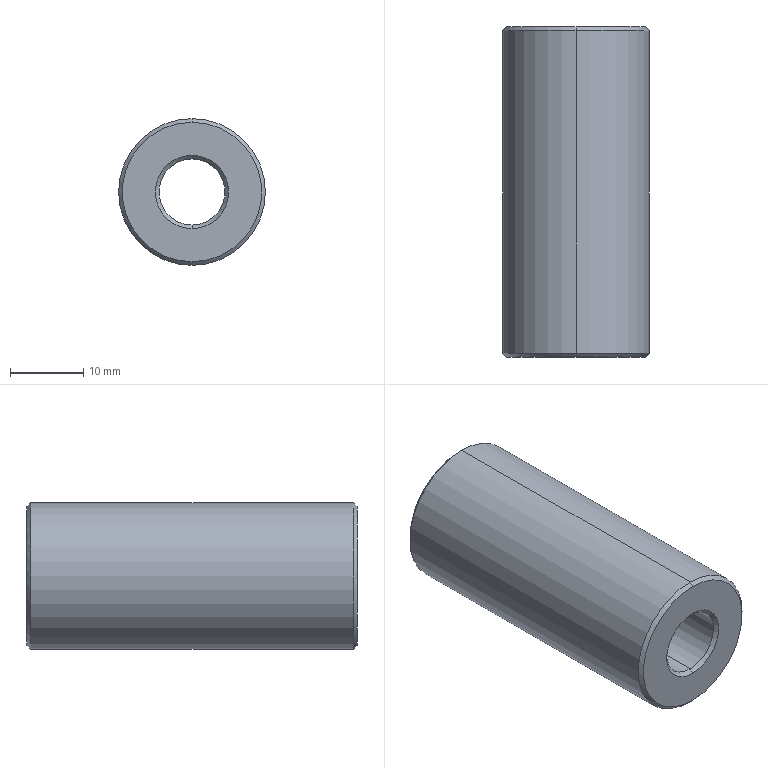Part | SolidWorks | features Chamfer 1, Extrusion 1, HoleWzd 1 | 1 solid | 17 faces | box 20 x 45 x 20 mm | volume 10277 mm3 | cone 8 | cylinder 6 | plane 3 | commonest cylinder face diameters 9 x2 15 x2 20 x2
STEP:
#1=CARTESIAN_POINT('',(0.,0.5,4.5));
#2=VERTEX_POINT('',#1);
#3=CARTESIAN_POINT('',(0.,0.5,-4.5));
#4=VERTEX_POINT('',#3);
#5=CARTESIAN_POINT('',(0.,0.5,0.));
#6=DIRECTION('',(0.,-1.,0.));
#7=DIRECTION('',(0.,0.,1.));
#8=AXIS2_PLACEMENT_3D('',#5,#6,#7);
#9=CIRCLE('',#8,4.5);
#10=EDGE_CURVE('',#2,#4,#9,.T.);
#11=ORIENTED_EDGE('',*,*,#10,.F.);
#12=CARTESIAN_POINT('',(0.,0.,5.));
#13=VERTEX_POINT('',#12);
#14=CARTESIAN_POINT('',(0.,0.,5.));
#15=DIRECTION('',(0.,-0.7071,0.7071));
#16=VECTOR('',#15,1000.);
#17=LINE('',#14,#16);
#18=EDGE_CURVE('',#2,#13,#17,.T.);
#19=ORIENTED_EDGE('',*,*,#18,.T.);
#20=CARTESIAN_POINT('',(0.,0.,-5.));
#21=VERTEX_POINT('',#20);
#22=CARTESIAN_POINT('',(0.,0.,0.));
#23=DIRECTION('',(0.,1.,0.));
#24=DIRECTION('',(0.,0.,1.));
#25=AXIS2_PLACEMENT_3D('',#22,#23,#24);
#26=CIRCLE('',#25,5.);
#27=EDGE_CURVE('',#21,#13,#26,.T.);
#28=ORIENTED_EDGE('',*,*,#27,.F.);
#29=CARTESIAN_POINT('',(0.,0.,-5.));
#30=DIRECTION('',(0.,-0.7071,-0.7071));
#31=VECTOR('',#30,1000.);
#32=LINE('',#29,#31);
#33=EDGE_CURVE('',#4,#21,#32,.T.);
#34=ORIENTED_EDGE('',*,*,#33,.F.);
#35=EDGE_LOOP('',(#11,#19,#28,#34));
#36=FACE_OUTER_BOUND('',#35,.T.);
#37=CARTESIAN_POINT('',(0.,0.,0.));
#38=DIRECTION('',(0.,-1.,0.));
#39=DIRECTION('',(0.,0.,-1.));
#40=AXIS2_PLACEMENT_3D('',#37,#38,#39);
#41=CONICAL_SURFACE('',#40,5.,0.7854);
#42=ADVANCED_FACE('',(#36),#41,.F.);
#43=CARTESIAN_POINT('',(0.,0.,-9.5));
#44=VERTEX_POINT('',#43);
#45=CARTESIAN_POINT('',(0.,0.,9.5));
#46=VERTEX_POINT('',#45);
#47=CARTESIAN_POINT('',(0.,0.,0.));
#48=DIRECTION('',(0.,-1.,0.));
#49=DIRECTION('',(0.,0.,1.));
#50=AXIS2_PLACEMENT_3D('',#47,#48,#49);
#51=CIRCLE('',#50,9.5);
#52=EDGE_CURVE('',#44,#46,#51,.T.);
#53=ORIENTED_EDGE('',*,*,#52,.F.);
#54=CARTESIAN_POINT('',(0.,0.5,-10.));
#55=VERTEX_POINT('',#54);
#56=CARTESIAN_POINT('',(0.,0.5,-10.));
#57=DIRECTION('',(0.,0.7071,-0.7071));
#58=VECTOR('',#57,1000.);
#59=LINE('',#56,#58);
#60=EDGE_CURVE('',#44,#55,#59,.T.);
#61=ORIENTED_EDGE('',*,*,#60,.T.);
#62=CARTESIAN_POINT('',(0.,0.5,10.));
#63=VERTEX_POINT('',#62);
#64=CARTESIAN_POINT('',(0.,0.5,0.));
#65=DIRECTION('',(0.,1.,0.));
#66=DIRECTION('',(0.,0.,1.));
#67=AXIS2_PLACEMENT_3D('',#64,#65,#66);
#68=CIRCLE('',#67,10.);
#69=EDGE_CURVE('',#63,#55,#68,.T.);
#70=ORIENTED_EDGE('',*,*,#69,.F.);
#71=CARTESIAN_POINT('',(0.,0.5,10.));
#72=DIRECTION('',(0.,0.7071,0.7071));
#73=VECTOR('',#72,1000.);
#74=LINE('',#71,#73);
#75=EDGE_CURVE('',#46,#63,#74,.T.);
#76=ORIENTED_EDGE('',*,*,#75,.F.);
#77=EDGE_LOOP('',(#53,#61,#70,#76));
#78=FACE_OUTER_BOUND('',#77,.T.);
#79=CARTESIAN_POINT('',(0.,0.5,0.));
#80=DIRECTION('',(0.,1.,0.));
#81=DIRECTION('',(0.,0.,1.));
#82=AXIS2_PLACEMENT_3D('',#79,#80,#81);
#83=CONICAL_SURFACE('',#82,10.,0.7854);
#84=ADVANCED_FACE('',(#78),#83,.T.);
#85=CARTESIAN_POINT('',(0.,44.5,-7.5));
#86=VERTEX_POINT('',#85);
#87=CARTESIAN_POINT('',(0.,44.5,7.5));
#88=VERTEX_POINT('',#87);
#89=CARTESIAN_POINT('',(0.,44.5,0.));
#90=DIRECTION('',(0.,1.,0.));
#91=DIRECTION('',(0.,0.,1.));
#92=AXIS2_PLACEMENT_3D('',#89,#90,#91);
#93=CIRCLE('',#92,7.5);
#94=EDGE_CURVE('',#86,#88,#93,.T.);
#95=ORIENTED_EDGE('',*,*,#94,.F.);
#96=CARTESIAN_POINT('',(0.,45.,-8.));
#97=VERTEX_POINT('',#96);
#98=CARTESIAN_POINT('',(0.,44.5,-7.5));
#99=DIRECTION('',(0.,0.7071,-0.7071));
#100=VECTOR('',#99,1000.);
#101=LINE('',#98,#100);
#102=EDGE_CURVE('',#86,#97,#101,.T.);
#103=ORIENTED_EDGE('',*,*,#102,.T.);
#104=CARTESIAN_POINT('',(0.,45.,8.));
#105=VERTEX_POINT('',#104);
#106=CARTESIAN_POINT('',(0.,45.,0.));
#107=DIRECTION('',(0.,-1.,0.));
#108=DIRECTION('',(0.,0.,1.));
#109=AXIS2_PLACEMENT_3D('',#106,#107,#108);
#110=CIRCLE('',#109,8.);
#111=EDGE_CURVE('',#105,#97,#110,.T.);
#112=ORIENTED_EDGE('',*,*,#111,.F.);
#113=CARTESIAN_POINT('',(0.,44.5,7.5));
#114=DIRECTION('',(0.,0.7071,0.7071));
#115=VECTOR('',#114,1000.);
#116=LINE('',#113,#115);
#117=EDGE_CURVE('',#88,#105,#116,.T.);
#118=ORIENTED_EDGE('',*,*,#117,.F.);
#119=EDGE_LOOP('',(#95,#103,#112,#118));
#120=FACE_OUTER_BOUND('',#119,.T.);
#121=CARTESIAN_POINT('',(0.,44.5,0.));
#122=DIRECTION('',(0.,1.,0.));
#123=DIRECTION('',(0.,0.,1.));
#124=AXIS2_PLACEMENT_3D('',#121,#122,#123);
#125=CONICAL_SURFACE('',#124,7.5,0.7854);
#126=ADVANCED_FACE('',(#120),#125,.F.);
#127=CARTESIAN_POINT('',(0.,45.,9.5));
#128=VERTEX_POINT('',#127);
#129=CARTESIAN_POINT('',(0.,45.,-9.5));
#130=VERTEX_POINT('',#129);
#131=CARTESIAN_POINT('',(0.,45.,0.));
#132=DIRECTION('',(0.,1.,0.));
#133=DIRECTION('',(0.,0.,1.));
#134=AXIS2_PLACEMENT_3D('',#131,#132,#133);
#135=CIRCLE('',#134,9.5);
#136=EDGE_CURVE('',#128,#130,#135,.T.);
#137=ORIENTED_EDGE('',*,*,#136,.F.);
#138=CARTESIAN_POINT('',(0.,44.5,10.));
#139=VERTEX_POINT('',#138);
#140=CARTESIAN_POINT('',(0.,45.,9.5));
#141=DIRECTION('',(0.,-0.7071,0.7071));
#142=VECTOR('',#141,1000.);
#143=LINE('',#140,#142);
#144=EDGE_CURVE('',#128,#139,#143,.T.);
#145=ORIENTED_EDGE('',*,*,#144,.T.);
#146=CARTESIAN_POINT('',(0.,44.5,-10.));
#147=VERTEX_POINT('',#146);
#148=CARTESIAN_POINT('',(0.,44.5,0.));
#149=DIRECTION('',(0.,-1.,0.));
#150=DIRECTION('',(0.,0.,1.));
#151=AXIS2_PLACEMENT_3D('',#148,#149,#150);
#152=CIRCLE('',#151,10.);
#153=EDGE_CURVE('',#147,#139,#152,.T.);
#154=ORIENTED_EDGE('',*,*,#153,.F.);
#155=CARTESIAN_POINT('',(0.,45.,-9.5));
#156=DIRECTION('',(0.,-0.7071,-0.7071));
#157=VECTOR('',#156,1000.);
#158=LINE('',#155,#157);
#159=EDGE_CURVE('',#130,#147,#158,.T.);
#160=ORIENTED_EDGE('',*,*,#159,.F.);
#161=EDGE_LOOP('',(#137,#145,#154,#160));
#162=FACE_OUTER_BOUND('',#161,.T.);
#163=CARTESIAN_POINT('',(0.,45.,0.));
#164=DIRECTION('',(0.,-1.,0.));
#165=DIRECTION('',(0.,0.,-1.));
#166=AXIS2_PLACEMENT_3D('',#163,#164,#165);
#167=CONICAL_SURFACE('',#166,9.5,0.7854);
#168=ADVANCED_FACE('',(#162),#167,.T.);
#169=CARTESIAN_POINT('',(0.,36.4,-7.5));
#170=VERTEX_POINT('',#169);
#171=CARTESIAN_POINT('',(0.,36.4,7.5));
#172=VERTEX_POINT('',#171);
#173=CARTESIAN_POINT('',(0.,36.4,0.));
#174=DIRECTION('',(0.,1.,0.));
#175=DIRECTION('',(0.,0.,1.));
#176=AXIS2_PLACEMENT_3D('',#173,#174,#175);
#177=CIRCLE('',#176,7.5);
#178=EDGE_CURVE('',#170,#172,#177,.T.);
#179=ORIENTED_EDGE('',*,*,#178,.F.);
#180=CARTESIAN_POINT('',(0.,45.,-7.5));
#181=DIRECTION('',(0.,1.,0.));
#182=VECTOR('',#181,1000.);
#183=LINE('',#180,#182);
#184=EDGE_CURVE('',#170,#86,#183,.T.);
#185=ORIENTED_EDGE('',*,*,#184,.T.);
#186=ORIENTED_EDGE('',*,*,#94,.T.);
#187=CARTESIAN_POINT('',(0.,45.,7.5));
#188=DIRECTION('',(0.,1.,0.));
#189=VECTOR('',#188,1000.);
#190=LINE('',#187,#189);
#191=EDGE_CURVE('',#172,#88,#190,.T.);
#192=ORIENTED_EDGE('',*,*,#191,.F.);
#193=EDGE_LOOP('',(#179,#185,#186,#192));
#194=FACE_OUTER_BOUND('',#193,.T.);
#195=CARTESIAN_POINT('',(0.,45.,0.));
#196=DIRECTION('',(0.,1.,0.));
#197=DIRECTION('',(0.,0.,1.));
#198=AXIS2_PLACEMENT_3D('',#195,#196,#197);
#199=CYLINDRICAL_SURFACE('',#198,7.5);
#200=ADVANCED_FACE('',(#194),#199,.F.);
#201=ORIENTED_EDGE('',*,*,#10,.T.);
#202=CARTESIAN_POINT('',(0.,36.4,-4.5));
#203=VERTEX_POINT('',#202);
#204=CARTESIAN_POINT('',(0.,45.,-4.5));
#205=DIRECTION('',(0.,1.,0.));
#206=VECTOR('',#205,1000.);
#207=LINE('',#204,#206);
#208=EDGE_CURVE('',#4,#203,#207,.T.);
#209=ORIENTED_EDGE('',*,*,#208,.T.);
#210=CARTESIAN_POINT('',(0.,36.4,4.5));
#211=VERTEX_POINT('',#210);
#212=CARTESIAN_POINT('',(0.,36.4,0.));
#213=DIRECTION('',(0.,1.,0.));
#214=DIRECTION('',(0.,0.,1.));
#215=AXIS2_PLACEMENT_3D('',#212,#213,#214);
#216=CIRCLE('',#215,4.5);
#217=EDGE_CURVE('',#203,#211,#216,.T.);
#218=ORIENTED_EDGE('',*,*,#217,.T.);
#219=CARTESIAN_POINT('',(0.,45.,4.5));
#220=DIRECTION('',(0.,1.,0.));
#221=VECTOR('',#220,1000.);
#222=LINE('',#219,#221);
#223=EDGE_CURVE('',#2,#211,#222,.T.);
#224=ORIENTED_EDGE('',*,*,#223,.F.);
#225=EDGE_LOOP('',(#201,#209,#218,#224));
#226=FACE_OUTER_BOUND('',#225,.T.);
#227=CARTESIAN_POINT('',(0.,45.,0.));
#228=DIRECTION('',(0.,1.,0.));
#229=DIRECTION('',(0.,0.,1.));
#230=AXIS2_PLACEMENT_3D('',#227,#228,#229);
#231=CYLINDRICAL_SURFACE('',#230,4.5);
#232=ADVANCED_FACE('',(#226),#231,.F.);
#233=ORIENTED_EDGE('',*,*,#153,.T.);
#234=CARTESIAN_POINT('',(0.,45.,10.));
#235=DIRECTION('',(0.,-1.,0.));
#236=VECTOR('',#235,1000.);
#237=LINE('',#234,#236);
#238=EDGE_CURVE('',#139,#63,#237,.T.);
#239=ORIENTED_EDGE('',*,*,#238,.T.);
#240=ORIENTED_EDGE('',*,*,#69,.T.);
#241=CARTESIAN_POINT('',(0.,45.,-10.));
#242=DIRECTION('',(0.,-1.,0.));
#243=VECTOR('',#242,1000.);
#244=LINE('',#241,#243);
#245=EDGE_CURVE('',#147,#55,#244,.T.);
#246=ORIENTED_EDGE('',*,*,#245,.F.);
#247=EDGE_LOOP('',(#233,#239,#240,#246));
#248=FACE_OUTER_BOUND('',#247,.T.);
#249=CARTESIAN_POINT('',(0.,45.,0.));
#250=DIRECTION('',(0.,-1.,0.));
#251=DIRECTION('',(0.,0.,-1.));
#252=AXIS2_PLACEMENT_3D('',#249,#250,#251);
#253=CYLINDRICAL_SURFACE('',#252,10.);
#254=ADVANCED_FACE('',(#248),#253,.T.);
#255=ORIENTED_EDGE('',*,*,#238,.F.);
#256=CARTESIAN_POINT('',(0.,44.5,0.));
#257=DIRECTION('',(0.,-1.,0.));
#258=DIRECTION('',(0.,0.,1.));
#259=AXIS2_PLACEMENT_3D('',#256,#257,#258);
#260=CIRCLE('',#259,10.);
#261=EDGE_CURVE('',#139,#147,#260,.T.);
#262=ORIENTED_EDGE('',*,*,#261,.T.);
#263=ORIENTED_EDGE('',*,*,#245,.T.);
#264=CARTESIAN_POINT('',(0.,0.5,0.));
#265=DIRECTION('',(0.,1.,0.));
#266=DIRECTION('',(0.,0.,1.));
#267=AXIS2_PLACEMENT_3D('',#264,#265,#266);
#268=CIRCLE('',#267,10.);
#269=EDGE_CURVE('',#55,#63,#268,.T.);
#270=ORIENTED_EDGE('',*,*,#269,.T.);
#271=EDGE_LOOP('',(#255,#262,#263,#270));
#272=FACE_OUTER_BOUND('',#271,.T.);
#273=CARTESIAN_POINT('',(0.,45.,0.));
#274=DIRECTION('',(0.,-1.,0.));
#275=DIRECTION('',(0.,0.,-1.));
#276=AXIS2_PLACEMENT_3D('',#273,#274,#275);
#277=CYLINDRICAL_SURFACE('',#276,10.);
#278=ADVANCED_FACE('',(#272),#277,.T.);
#279=CARTESIAN_POINT('',(0.,45.,0.));
#280=DIRECTION('',(0.,1.,0.));
#281=DIRECTION('',(0.,0.,1.));
#282=AXIS2_PLACEMENT_3D('',#279,#280,#281);
#283=CIRCLE('',#282,9.5);
#284=EDGE_CURVE('',#130,#128,#283,.T.);
#285=ORIENTED_EDGE('',*,*,#284,.T.);
#286=ORIENTED_EDGE('',*,*,#136,.T.);
#287=EDGE_LOOP('',(#285,#286));
#288=FACE_OUTER_BOUND('',#287,.T.);
#289=ORIENTED_EDGE('',*,*,#111,.T.);
#290=CARTESIAN_POINT('',(0.,45.,0.));
#291=DIRECTION('',(0.,-1.,0.));
#292=DIRECTION('',(0.,0.,1.));
#293=AXIS2_PLACEMENT_3D('',#290,#291,#292);
#294=CIRCLE('',#293,8.);
#295=EDGE_CURVE('',#97,#105,#294,.T.);
#296=ORIENTED_EDGE('',*,*,#295,.T.);
#297=EDGE_LOOP('',(#289,#296));
#298=FACE_BOUND('',#297,.T.);
#299=CARTESIAN_POINT('',(0.,45.,0.));
#300=DIRECTION('',(0.,1.,0.));
#301=DIRECTION('',(0.,0.,1.));
#302=AXIS2_PLACEMENT_3D('',#299,#300,#301);
#303=PLANE('',#302);
#304=ADVANCED_FACE('',(#288,#298),#303,.T.);
#305=CARTESIAN_POINT('',(0.,0.,0.));
#306=DIRECTION('',(0.,-1.,0.));
#307=DIRECTION('',(0.,0.,1.));
#308=AXIS2_PLACEMENT_3D('',#305,#306,#307);
#309=CIRCLE('',#308,9.5);
#310=EDGE_CURVE('',#46,#44,#309,.T.);
#311=ORIENTED_EDGE('',*,*,#310,.T.);
#312=ORIENTED_EDGE('',*,*,#52,.T.);
#313=EDGE_LOOP('',(#311,#312));
#314=FACE_OUTER_BOUND('',#313,.T.);
#315=ORIENTED_EDGE('',*,*,#27,.T.);
#316=CARTESIAN_POINT('',(0.,0.,0.));
#317=DIRECTION('',(0.,1.,0.));
#318=DIRECTION('',(0.,0.,1.));
#319=AXIS2_PLACEMENT_3D('',#316,#317,#318);
#320=CIRCLE('',#319,5.);
#321=EDGE_CURVE('',#13,#21,#320,.T.);
#322=ORIENTED_EDGE('',*,*,#321,.T.);
#323=EDGE_LOOP('',(#315,#322));
#324=FACE_BOUND('',#323,.T.);
#325=CARTESIAN_POINT('',(0.,0.,0.));
#326=DIRECTION('',(0.,1.,0.));
#327=DIRECTION('',(0.,0.,1.));
#328=AXIS2_PLACEMENT_3D('',#325,#326,#327);
#329=PLANE('',#328);
#330=ADVANCED_FACE('',(#314,#324),#329,.F.);
#331=ORIENTED_EDGE('',*,*,#208,.F.);
#332=CARTESIAN_POINT('',(0.,0.5,0.));
#333=DIRECTION('',(0.,-1.,0.));
#334=DIRECTION('',(0.,0.,1.));
#335=AXIS2_PLACEMENT_3D('',#332,#333,#334);
#336=CIRCLE('',#335,4.5);
#337=EDGE_CURVE('',#4,#2,#336,.T.);
#338=ORIENTED_EDGE('',*,*,#337,.T.);
#339=ORIENTED_EDGE('',*,*,#223,.T.);
#340=CARTESIAN_POINT('',(0.,36.4,0.));
#341=DIRECTION('',(0.,1.,0.));
#342=DIRECTION('',(0.,0.,1.));
#343=AXIS2_PLACEMENT_3D('',#340,#341,#342);
#344=CIRCLE('',#343,4.5);
#345=EDGE_CURVE('',#211,#203,#344,.T.);
#346=ORIENTED_EDGE('',*,*,#345,.T.);
#347=EDGE_LOOP('',(#331,#338,#339,#346));
#348=FACE_OUTER_BOUND('',#347,.T.);
#349=CARTESIAN_POINT('',(0.,45.,0.));
#350=DIRECTION('',(0.,1.,0.));
#351=DIRECTION('',(0.,0.,1.));
#352=AXIS2_PLACEMENT_3D('',#349,#350,#351);
#353=CYLINDRICAL_SURFACE('',#352,4.5);
#354=ADVANCED_FACE('',(#348),#353,.F.);
#355=ORIENTED_EDGE('',*,*,#345,.F.);
#356=ORIENTED_EDGE('',*,*,#217,.F.);
#357=EDGE_LOOP('',(#355,#356));
#358=FACE_BOUND('',#357,.T.);
#359=CARTESIAN_POINT('',(0.,36.4,0.));
#360=DIRECTION('',(0.,1.,0.));
#361=DIRECTION('',(0.,0.,1.));
#362=AXIS2_PLACEMENT_3D('',#359,#360,#361);
#363=CIRCLE('',#362,7.5);
#364=EDGE_CURVE('',#172,#170,#363,.T.);
#365=ORIENTED_EDGE('',*,*,#364,.T.);
#366=ORIENTED_EDGE('',*,*,#178,.T.);
#367=EDGE_LOOP('',(#365,#366));
#368=FACE_OUTER_BOUND('',#367,.T.);
#369=CARTESIAN_POINT('',(4.5,36.4,0.));
#370=DIRECTION('',(0.,-1.,0.));
#371=DIRECTION('',(0.,0.,-1.));
#372=AXIS2_PLACEMENT_3D('',#369,#370,#371);
#373=PLANE('',#372);
#374=ADVANCED_FACE('',(#358,#368),#373,.F.);
#375=ORIENTED_EDGE('',*,*,#184,.F.);
#376=ORIENTED_EDGE('',*,*,#364,.F.);
#377=ORIENTED_EDGE('',*,*,#191,.T.);
#378=CARTESIAN_POINT('',(0.,44.5,0.));
#379=DIRECTION('',(0.,1.,0.));
#380=DIRECTION('',(0.,0.,1.));
#381=AXIS2_PLACEMENT_3D('',#378,#379,#380);
#382=CIRCLE('',#381,7.5);
#383=EDGE_CURVE('',#88,#86,#382,.T.);
#384=ORIENTED_EDGE('',*,*,#383,.T.);
#385=EDGE_LOOP('',(#375,#376,#377,#384));
#386=FACE_OUTER_BOUND('',#385,.T.);
#387=CARTESIAN_POINT('',(0.,45.,0.));
#388=DIRECTION('',(0.,1.,0.));
#389=DIRECTION('',(0.,0.,1.));
#390=AXIS2_PLACEMENT_3D('',#387,#388,#389);
#391=CYLINDRICAL_SURFACE('',#390,7.5);
#392=ADVANCED_FACE('',(#386),#391,.F.);
#393=ORIENTED_EDGE('',*,*,#144,.F.);
#394=ORIENTED_EDGE('',*,*,#284,.F.);
#395=ORIENTED_EDGE('',*,*,#159,.T.);
#396=ORIENTED_EDGE('',*,*,#261,.F.);
#397=EDGE_LOOP('',(#393,#394,#395,#396));
#398=FACE_OUTER_BOUND('',#397,.T.);
#399=CARTESIAN_POINT('',(0.,45.,0.));
#400=DIRECTION('',(0.,-1.,0.));
#401=DIRECTION('',(0.,0.,-1.));
#402=AXIS2_PLACEMENT_3D('',#399,#400,#401);
#403=CONICAL_SURFACE('',#402,9.5,0.7854);
#404=ADVANCED_FACE('',(#398),#403,.T.);
#405=ORIENTED_EDGE('',*,*,#102,.F.);
#406=ORIENTED_EDGE('',*,*,#383,.F.);
#407=ORIENTED_EDGE('',*,*,#117,.T.);
#408=ORIENTED_EDGE('',*,*,#295,.F.);
#409=EDGE_LOOP('',(#405,#406,#407,#408));
#410=FACE_OUTER_BOUND('',#409,.T.);
#411=CARTESIAN_POINT('',(0.,44.5,0.));
#412=DIRECTION('',(0.,1.,0.));
#413=DIRECTION('',(0.,0.,1.));
#414=AXIS2_PLACEMENT_3D('',#411,#412,#413);
#415=CONICAL_SURFACE('',#414,7.5,0.7854);
#416=ADVANCED_FACE('',(#410),#415,.F.);
#417=ORIENTED_EDGE('',*,*,#60,.F.);
#418=ORIENTED_EDGE('',*,*,#310,.F.);
#419=ORIENTED_EDGE('',*,*,#75,.T.);
#420=ORIENTED_EDGE('',*,*,#269,.F.);
#421=EDGE_LOOP('',(#417,#418,#419,#420));
#422=FACE_OUTER_BOUND('',#421,.T.);
#423=CARTESIAN_POINT('',(0.,0.5,0.));
#424=DIRECTION('',(0.,1.,0.));
#425=DIRECTION('',(0.,0.,1.));
#426=AXIS2_PLACEMENT_3D('',#423,#424,#425);
#427=CONICAL_SURFACE('',#426,10.,0.7854);
#428=ADVANCED_FACE('',(#422),#427,.T.);
#429=ORIENTED_EDGE('',*,*,#18,.F.);
#430=ORIENTED_EDGE('',*,*,#337,.F.);
#431=ORIENTED_EDGE('',*,*,#33,.T.);
#432=ORIENTED_EDGE('',*,*,#321,.F.);
#433=EDGE_LOOP('',(#429,#430,#431,#432));
#434=FACE_OUTER_BOUND('',#433,.T.);
#435=CARTESIAN_POINT('',(0.,0.,0.));
#436=DIRECTION('',(0.,-1.,0.));
#437=DIRECTION('',(0.,0.,-1.));
#438=AXIS2_PLACEMENT_3D('',#435,#436,#437);
#439=CONICAL_SURFACE('',#438,5.,0.7854);
#440=ADVANCED_FACE('',(#434),#439,.F.);
#441=CLOSED_SHELL('',(#42,#84,#126,#168,#200,#232,#254,#278,#304,#330,#354,#374,#392,#404,#416,#428,#440));
#442=MANIFOLD_SOLID_BREP('',#441);
#443=CARTESIAN_POINT('',(0.,0.,0.));
#444=DIRECTION('',(0.,0.,1.));
#445=DIRECTION('',(1.,0.,0.));
#446=AXIS2_PLACEMENT_3D('',#443,#444,#445);
#447=(LENGTH_UNIT()NAMED_UNIT(*)SI_UNIT(.MILLI.,.METRE.));
#448=UNCERTAINTY_MEASURE_WITH_UNIT(LENGTH_MEASURE(0.00001),#447,'','');
#449=(NAMED_UNIT(*)PLANE_ANGLE_UNIT()SI_UNIT($,.RADIAN.));
#450=(NAMED_UNIT(*)SI_UNIT($,.STERADIAN.)SOLID_ANGLE_UNIT());
#451=(GEOMETRIC_REPRESENTATION_CONTEXT(3)GLOBAL_UNCERTAINTY_ASSIGNED_CONTEXT((#448))GLOBAL_UNIT_ASSIGNED_CONTEXT((#447,#449,#450))REPRESENTATION_CONTEXT('',''));
#452=ADVANCED_BREP_SHAPE_REPRESENTATION('',(#442,#446),#451);